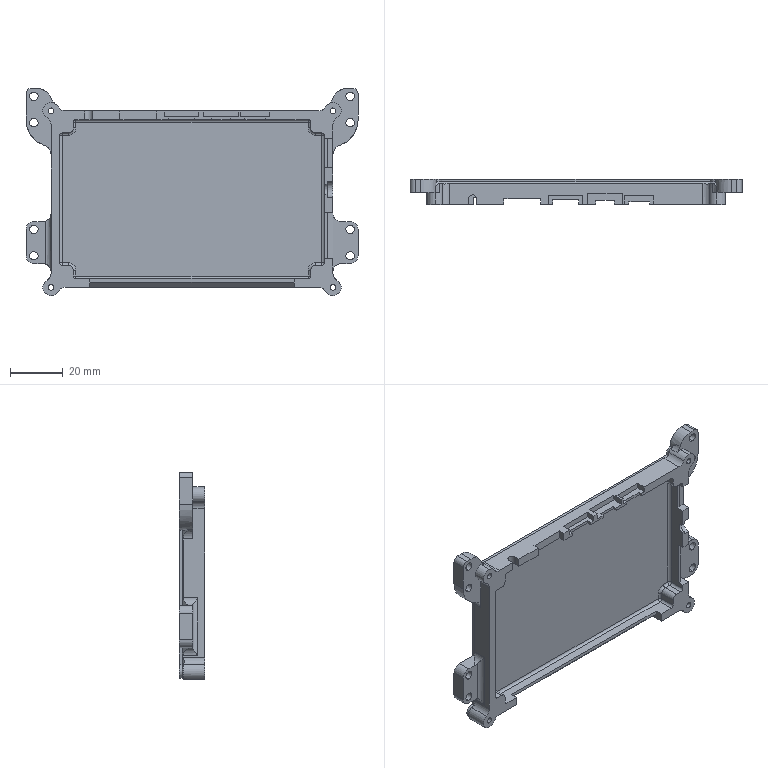Part | SolidWorks | features Fillet 7, ICE 4, Cut 2, MBimport 1, MirrorPattern 1 | 1 solid | 217 faces | box 126 x 9.5 x 78.6 mm | volume 28044 mm3 | cylinder 100 | plane 97 | sphere 8 | cone 8 | torus 4 | commonest cylinder face diameters 2 x20 3.2 x17 6 x17 4 x9 2.2 x8 5.2 x8